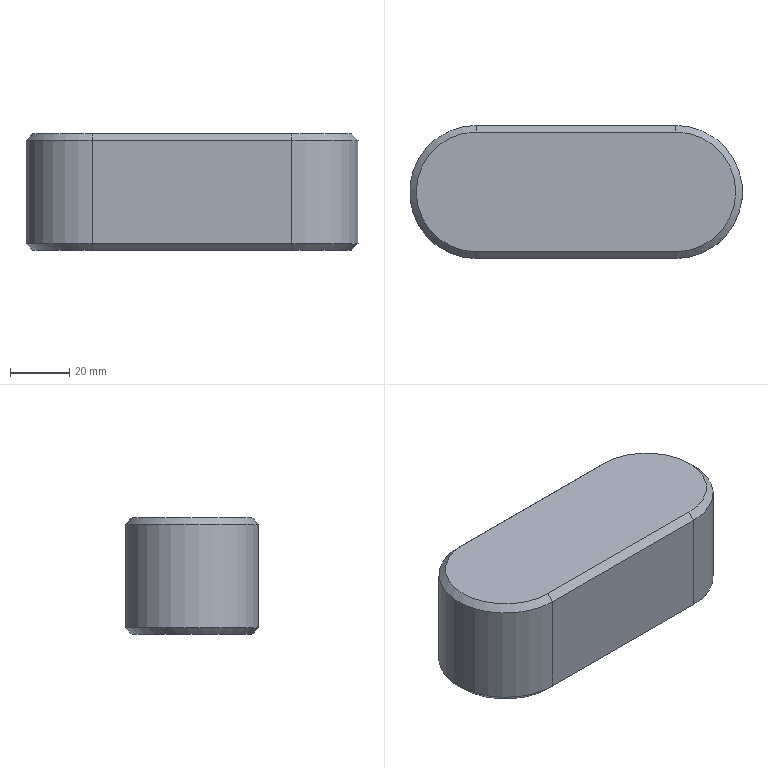Part | NX | features 28.SLDPRT 2, Delete Body 1, LINKED_BODY 1, SCALE 1 | 1 solid | 14 faces | box 112.5 x 45 x 39.375 mm | volume 180850 mm3 | plane 8 | cone 4 | cylinder 2 | commonest cylinder face diameters 45 x2
STEP:
#1=CARTESIAN_POINT('',(-34.875,-1747.479,329.645));
#2=VERTEX_POINT('',#1);
#3=CARTESIAN_POINT('',(-34.875,-1747.479,294.77));
#4=VERTEX_POINT('',#3);
#5=CARTESIAN_POINT('',(-34.875,-1747.479,331.895));
#6=DIRECTION('',(0.,0.,-1.));
#7=VECTOR('',#6,1000.);
#8=LINE('',#5,#7);
#9=EDGE_CURVE('',#2,#4,#8,.T.);
#10=ORIENTED_EDGE('',*,*,#9,.F.);
#11=CARTESIAN_POINT('',(-34.875,-1702.479,329.645));
#12=VERTEX_POINT('',#11);
#13=CARTESIAN_POINT('',(-34.875,-1724.979,329.645));
#14=DIRECTION('',(0.,0.,-1.));
#15=DIRECTION('',(-1.,0.,0.));
#16=AXIS2_PLACEMENT_3D('',#13,#14,#15);
#17=CIRCLE('',#16,22.5);
#18=EDGE_CURVE('',#2,#12,#17,.T.);
#19=ORIENTED_EDGE('',*,*,#18,.T.);
#20=CARTESIAN_POINT('',(-34.875,-1702.479,294.77));
#21=VERTEX_POINT('',#20);
#22=CARTESIAN_POINT('',(-34.875,-1702.479,331.895));
#23=DIRECTION('',(0.,0.,-1.));
#24=VECTOR('',#23,1000.);
#25=LINE('',#22,#24);
#26=EDGE_CURVE('',#12,#21,#25,.T.);
#27=ORIENTED_EDGE('',*,*,#26,.T.);
#28=CARTESIAN_POINT('',(-34.875,-1724.979,294.77));
#29=DIRECTION('',(0.,0.,-1.));
#30=DIRECTION('',(-1.,0.,0.));
#31=AXIS2_PLACEMENT_3D('',#28,#29,#30);
#32=CIRCLE('',#31,22.5);
#33=EDGE_CURVE('',#21,#4,#32,.F.);
#34=ORIENTED_EDGE('',*,*,#33,.T.);
#35=EDGE_LOOP('',(#10,#19,#27,#34));
#36=FACE_BOUND('',#35,.T.);
#37=CARTESIAN_POINT('',(-34.875,-1724.979,331.895));
#38=DIRECTION('',(0.,0.,-1.));
#39=DIRECTION('',(-1.,0.,0.));
#40=AXIS2_PLACEMENT_3D('',#37,#38,#39);
#41=CYLINDRICAL_SURFACE('',#40,22.5);
#42=ADVANCED_FACE('',(#36),#41,.T.);
#43=ORIENTED_EDGE('',*,*,#9,.T.);
#44=CARTESIAN_POINT('',(32.625,-1747.479,294.77));
#45=VERTEX_POINT('',#44);
#46=CARTESIAN_POINT('',(32.625,-1747.479,294.77));
#47=DIRECTION('',(1.,0.,0.));
#48=VECTOR('',#47,1000.);
#49=LINE('',#46,#48);
#50=EDGE_CURVE('',#4,#45,#49,.T.);
#51=ORIENTED_EDGE('',*,*,#50,.T.);
#52=CARTESIAN_POINT('',(32.625,-1747.479,329.645));
#53=VERTEX_POINT('',#52);
#54=CARTESIAN_POINT('',(32.625,-1747.479,331.895));
#55=DIRECTION('',(0.,0.,-1.));
#56=VECTOR('',#55,1000.);
#57=LINE('',#54,#56);
#58=EDGE_CURVE('',#53,#45,#57,.T.);
#59=ORIENTED_EDGE('',*,*,#58,.F.);
#60=CARTESIAN_POINT('',(32.625,-1747.479,329.645));
#61=DIRECTION('',(-1.,0.,0.));
#62=VECTOR('',#61,1000.);
#63=LINE('',#60,#62);
#64=EDGE_CURVE('',#53,#2,#63,.T.);
#65=ORIENTED_EDGE('',*,*,#64,.T.);
#66=EDGE_LOOP('',(#43,#51,#59,#65));
#67=FACE_BOUND('',#66,.T.);
#68=CARTESIAN_POINT('',(32.625,-1747.479,331.895));
#69=DIRECTION('',(0.,1.,0.));
#70=DIRECTION('',(-1.,0.,0.));
#71=AXIS2_PLACEMENT_3D('',#68,#69,#70);
#72=PLANE('',#71);
#73=ADVANCED_FACE('',(#67),#72,.F.);
#74=CARTESIAN_POINT('',(32.625,-1702.479,329.645));
#75=VERTEX_POINT('',#74);
#76=CARTESIAN_POINT('',(32.625,-1702.479,294.77));
#77=VERTEX_POINT('',#76);
#78=CARTESIAN_POINT('',(32.625,-1702.479,331.895));
#79=DIRECTION('',(0.,0.,-1.));
#80=VECTOR('',#79,1000.);
#81=LINE('',#78,#80);
#82=EDGE_CURVE('',#75,#77,#81,.T.);
#83=ORIENTED_EDGE('',*,*,#82,.F.);
#84=CARTESIAN_POINT('',(32.625,-1724.979,329.645));
#85=DIRECTION('',(0.,0.,-1.));
#86=DIRECTION('',(-1.,0.,0.));
#87=AXIS2_PLACEMENT_3D('',#84,#85,#86);
#88=CIRCLE('',#87,22.5);
#89=EDGE_CURVE('',#75,#53,#88,.T.);
#90=ORIENTED_EDGE('',*,*,#89,.T.);
#91=ORIENTED_EDGE('',*,*,#58,.T.);
#92=CARTESIAN_POINT('',(32.625,-1724.979,294.77));
#93=DIRECTION('',(0.,0.,-1.));
#94=DIRECTION('',(-1.,0.,0.));
#95=AXIS2_PLACEMENT_3D('',#92,#93,#94);
#96=CIRCLE('',#95,22.5);
#97=EDGE_CURVE('',#45,#77,#96,.F.);
#98=ORIENTED_EDGE('',*,*,#97,.T.);
#99=EDGE_LOOP('',(#83,#90,#91,#98));
#100=FACE_BOUND('',#99,.T.);
#101=CARTESIAN_POINT('',(32.625,-1724.979,331.895));
#102=DIRECTION('',(0.,0.,-1.));
#103=DIRECTION('',(-1.,0.,0.));
#104=AXIS2_PLACEMENT_3D('',#101,#102,#103);
#105=CYLINDRICAL_SURFACE('',#104,22.5);
#106=ADVANCED_FACE('',(#100),#105,.T.);
#107=ORIENTED_EDGE('',*,*,#26,.F.);
#108=CARTESIAN_POINT('',(-34.875,-1702.479,329.645));
#109=DIRECTION('',(1.,0.,0.));
#110=VECTOR('',#109,1000.);
#111=LINE('',#108,#110);
#112=EDGE_CURVE('',#12,#75,#111,.T.);
#113=ORIENTED_EDGE('',*,*,#112,.T.);
#114=ORIENTED_EDGE('',*,*,#82,.T.);
#115=CARTESIAN_POINT('',(-34.875,-1702.479,294.77));
#116=DIRECTION('',(-1.,0.,0.));
#117=VECTOR('',#116,1000.);
#118=LINE('',#115,#117);
#119=EDGE_CURVE('',#77,#21,#118,.T.);
#120=ORIENTED_EDGE('',*,*,#119,.T.);
#121=EDGE_LOOP('',(#107,#113,#114,#120));
#122=FACE_BOUND('',#121,.T.);
#123=CARTESIAN_POINT('',(-34.875,-1702.479,331.895));
#124=DIRECTION('',(0.,-1.,0.));
#125=DIRECTION('',(0.,0.,-1.));
#126=AXIS2_PLACEMENT_3D('',#123,#124,#125);
#127=PLANE('',#126);
#128=ADVANCED_FACE('',(#122),#127,.F.);
#129=CARTESIAN_POINT('',(-34.875,-1704.729,331.895));
#130=VERTEX_POINT('',#129);
#131=CARTESIAN_POINT('',(-34.875,-1745.229,331.895));
#132=VERTEX_POINT('',#131);
#133=CARTESIAN_POINT('',(-34.875,-1724.979,331.895));
#134=DIRECTION('',(0.,0.,-1.));
#135=DIRECTION('',(-1.,0.,0.));
#136=AXIS2_PLACEMENT_3D('',#133,#134,#135);
#137=CIRCLE('',#136,20.25);
#138=EDGE_CURVE('',#130,#132,#137,.F.);
#139=ORIENTED_EDGE('',*,*,#138,.T.);
#140=CARTESIAN_POINT('',(32.625,-1745.229,331.895));
#141=VERTEX_POINT('',#140);
#142=CARTESIAN_POINT('',(-34.875,-1745.229,331.895));
#143=DIRECTION('',(1.,0.,0.));
#144=VECTOR('',#143,1000.);
#145=LINE('',#142,#144);
#146=EDGE_CURVE('',#132,#141,#145,.T.);
#147=ORIENTED_EDGE('',*,*,#146,.T.);
#148=CARTESIAN_POINT('',(32.625,-1704.729,331.895));
#149=VERTEX_POINT('',#148);
#150=CARTESIAN_POINT('',(32.625,-1724.979,331.895));
#151=DIRECTION('',(0.,0.,-1.));
#152=DIRECTION('',(-1.,0.,0.));
#153=AXIS2_PLACEMENT_3D('',#150,#151,#152);
#154=CIRCLE('',#153,20.25);
#155=EDGE_CURVE('',#141,#149,#154,.F.);
#156=ORIENTED_EDGE('',*,*,#155,.T.);
#157=CARTESIAN_POINT('',(-34.875,-1704.729,331.895));
#158=DIRECTION('',(-1.,0.,0.));
#159=VECTOR('',#158,1000.);
#160=LINE('',#157,#159);
#161=EDGE_CURVE('',#149,#130,#160,.T.);
#162=ORIENTED_EDGE('',*,*,#161,.T.);
#163=EDGE_LOOP('',(#139,#147,#156,#162));
#164=FACE_BOUND('',#163,.T.);
#165=CARTESIAN_POINT('',(-34.875,-1724.979,331.895));
#166=DIRECTION('',(0.,0.,-1.));
#167=DIRECTION('',(-1.,0.,0.));
#168=AXIS2_PLACEMENT_3D('',#165,#166,#167);
#169=PLANE('',#168);
#170=ADVANCED_FACE('',(#164),#169,.F.);
#171=CARTESIAN_POINT('',(32.625,-1704.729,292.52));
#172=VERTEX_POINT('',#171);
#173=CARTESIAN_POINT('',(32.625,-1745.229,292.52));
#174=VERTEX_POINT('',#173);
#175=CARTESIAN_POINT('',(32.625,-1724.979,292.52));
#176=DIRECTION('',(0.,0.,-1.));
#177=DIRECTION('',(-1.,0.,0.));
#178=AXIS2_PLACEMENT_3D('',#175,#176,#177);
#179=CIRCLE('',#178,20.25);
#180=EDGE_CURVE('',#172,#174,#179,.T.);
#181=ORIENTED_EDGE('',*,*,#180,.T.);
#182=CARTESIAN_POINT('',(-34.875,-1745.229,292.52));
#183=VERTEX_POINT('',#182);
#184=CARTESIAN_POINT('',(-34.875,-1745.229,292.52));
#185=DIRECTION('',(-1.,0.,0.));
#186=VECTOR('',#185,1000.);
#187=LINE('',#184,#186);
#188=EDGE_CURVE('',#174,#183,#187,.T.);
#189=ORIENTED_EDGE('',*,*,#188,.T.);
#190=CARTESIAN_POINT('',(-34.875,-1704.729,292.52));
#191=VERTEX_POINT('',#190);
#192=CARTESIAN_POINT('',(-34.875,-1724.979,292.52));
#193=DIRECTION('',(0.,0.,-1.));
#194=DIRECTION('',(-1.,0.,0.));
#195=AXIS2_PLACEMENT_3D('',#192,#193,#194);
#196=CIRCLE('',#195,20.25);
#197=EDGE_CURVE('',#183,#191,#196,.T.);
#198=ORIENTED_EDGE('',*,*,#197,.T.);
#199=CARTESIAN_POINT('',(32.625,-1704.729,292.52));
#200=DIRECTION('',(1.,0.,0.));
#201=VECTOR('',#200,1000.);
#202=LINE('',#199,#201);
#203=EDGE_CURVE('',#191,#172,#202,.T.);
#204=ORIENTED_EDGE('',*,*,#203,.T.);
#205=EDGE_LOOP('',(#181,#189,#198,#204));
#206=FACE_BOUND('',#205,.T.);
#207=CARTESIAN_POINT('',(-34.875,-1724.979,292.52));
#208=DIRECTION('',(0.,0.,-1.));
#209=DIRECTION('',(-1.,0.,0.));
#210=AXIS2_PLACEMENT_3D('',#207,#208,#209);
#211=PLANE('',#210);
#212=ADVANCED_FACE('',(#206),#211,.T.);
#213=CARTESIAN_POINT('',(32.625,-1704.729,292.52));
#214=DIRECTION('',(0.,0.7071,0.7071));
#215=VECTOR('',#214,1000.);
#216=LINE('',#213,#215);
#217=EDGE_CURVE('',#172,#77,#216,.T.);
#218=ORIENTED_EDGE('',*,*,#217,.F.);
#219=ORIENTED_EDGE('',*,*,#203,.F.);
#220=CARTESIAN_POINT('',(-34.875,-1702.479,294.77));
#221=DIRECTION('',(0.,-0.7071,-0.7071));
#222=VECTOR('',#221,1000.);
#223=LINE('',#220,#222);
#224=EDGE_CURVE('',#21,#191,#223,.T.);
#225=ORIENTED_EDGE('',*,*,#224,.F.);
#226=ORIENTED_EDGE('',*,*,#119,.F.);
#227=EDGE_LOOP('',(#218,#219,#225,#226));
#228=FACE_BOUND('',#227,.T.);
#229=CARTESIAN_POINT('',(-34.875,-1702.479,294.77));
#230=DIRECTION('',(0.,0.7071,-0.7071));
#231=DIRECTION('',(0.,0.7071,0.7071));
#232=AXIS2_PLACEMENT_3D('',#229,#230,#231);
#233=PLANE('',#232);
#234=ADVANCED_FACE('',(#228),#233,.T.);
#235=ORIENTED_EDGE('',*,*,#224,.T.);
#236=ORIENTED_EDGE('',*,*,#197,.F.);
#237=CARTESIAN_POINT('',(-34.875,-1747.479,294.77));
#238=DIRECTION('',(0.,0.7071,-0.7071));
#239=VECTOR('',#238,1000.);
#240=LINE('',#237,#239);
#241=EDGE_CURVE('',#4,#183,#240,.T.);
#242=ORIENTED_EDGE('',*,*,#241,.F.);
#243=ORIENTED_EDGE('',*,*,#33,.F.);
#244=EDGE_LOOP('',(#235,#236,#242,#243));
#245=FACE_BOUND('',#244,.T.);
#246=CARTESIAN_POINT('',(-34.875,-1724.979,294.77));
#247=DIRECTION('',(0.,0.,1.));
#248=DIRECTION('',(1.,0.,0.));
#249=AXIS2_PLACEMENT_3D('',#246,#247,#248);
#250=CONICAL_SURFACE('',#249,22.5,0.7854);
#251=ADVANCED_FACE('',(#245),#250,.T.);
#252=ORIENTED_EDGE('',*,*,#217,.T.);
#253=ORIENTED_EDGE('',*,*,#97,.F.);
#254=CARTESIAN_POINT('',(32.625,-1745.229,292.52));
#255=DIRECTION('',(0.,-0.7071,0.7071));
#256=VECTOR('',#255,1000.);
#257=LINE('',#254,#256);
#258=EDGE_CURVE('',#174,#45,#257,.T.);
#259=ORIENTED_EDGE('',*,*,#258,.F.);
#260=ORIENTED_EDGE('',*,*,#180,.F.);
#261=EDGE_LOOP('',(#252,#253,#259,#260));
#262=FACE_BOUND('',#261,.T.);
#263=CARTESIAN_POINT('',(32.625,-1724.979,294.77));
#264=DIRECTION('',(0.,0.,1.));
#265=DIRECTION('',(1.,0.,0.));
#266=AXIS2_PLACEMENT_3D('',#263,#264,#265);
#267=CONICAL_SURFACE('',#266,22.5,0.7854);
#268=ADVANCED_FACE('',(#262),#267,.T.);
#269=ORIENTED_EDGE('',*,*,#241,.T.);
#270=ORIENTED_EDGE('',*,*,#188,.F.);
#271=ORIENTED_EDGE('',*,*,#258,.T.);
#272=ORIENTED_EDGE('',*,*,#50,.F.);
#273=EDGE_LOOP('',(#269,#270,#271,#272));
#274=FACE_BOUND('',#273,.T.);
#275=CARTESIAN_POINT('',(32.625,-1747.479,294.77));
#276=DIRECTION('',(0.,-0.7071,-0.7071));
#277=DIRECTION('',(0.,0.7071,-0.7071));
#278=AXIS2_PLACEMENT_3D('',#275,#276,#277);
#279=PLANE('',#278);
#280=ADVANCED_FACE('',(#274),#279,.T.);
#281=CARTESIAN_POINT('',(32.625,-1702.479,329.645));
#282=DIRECTION('',(0.,-0.7071,0.7071));
#283=VECTOR('',#282,1000.);
#284=LINE('',#281,#283);
#285=EDGE_CURVE('',#75,#149,#284,.T.);
#286=ORIENTED_EDGE('',*,*,#285,.F.);
#287=ORIENTED_EDGE('',*,*,#112,.F.);
#288=CARTESIAN_POINT('',(-34.875,-1704.729,331.895));
#289=DIRECTION('',(0.,0.7071,-0.7071));
#290=VECTOR('',#289,1000.);
#291=LINE('',#288,#290);
#292=EDGE_CURVE('',#130,#12,#291,.T.);
#293=ORIENTED_EDGE('',*,*,#292,.F.);
#294=ORIENTED_EDGE('',*,*,#161,.F.);
#295=EDGE_LOOP('',(#286,#287,#293,#294));
#296=FACE_BOUND('',#295,.T.);
#297=CARTESIAN_POINT('',(-34.875,-1704.729,331.895));
#298=DIRECTION('',(0.,-0.7071,-0.7071));
#299=DIRECTION('',(0.,0.7071,-0.7071));
#300=AXIS2_PLACEMENT_3D('',#297,#298,#299);
#301=PLANE('',#300);
#302=ADVANCED_FACE('',(#296),#301,.F.);
#303=ORIENTED_EDGE('',*,*,#292,.T.);
#304=ORIENTED_EDGE('',*,*,#18,.F.);
#305=CARTESIAN_POINT('',(-34.875,-1745.229,331.895));
#306=DIRECTION('',(0.,-0.7071,-0.7071));
#307=VECTOR('',#306,1000.);
#308=LINE('',#305,#307);
#309=EDGE_CURVE('',#132,#2,#308,.T.);
#310=ORIENTED_EDGE('',*,*,#309,.F.);
#311=ORIENTED_EDGE('',*,*,#138,.F.);
#312=EDGE_LOOP('',(#303,#304,#310,#311));
#313=FACE_BOUND('',#312,.T.);
#314=CARTESIAN_POINT('',(-34.875,-1724.979,331.895));
#315=DIRECTION('',(0.,0.,-1.));
#316=DIRECTION('',(-1.,0.,0.));
#317=AXIS2_PLACEMENT_3D('',#314,#315,#316);
#318=CONICAL_SURFACE('',#317,20.25,0.7854);
#319=ADVANCED_FACE('',(#313),#318,.T.);
#320=ORIENTED_EDGE('',*,*,#285,.T.);
#321=ORIENTED_EDGE('',*,*,#155,.F.);
#322=CARTESIAN_POINT('',(32.625,-1747.479,329.645));
#323=DIRECTION('',(0.,0.7071,0.7071));
#324=VECTOR('',#323,1000.);
#325=LINE('',#322,#324);
#326=EDGE_CURVE('',#53,#141,#325,.T.);
#327=ORIENTED_EDGE('',*,*,#326,.F.);
#328=ORIENTED_EDGE('',*,*,#89,.F.);
#329=EDGE_LOOP('',(#320,#321,#327,#328));
#330=FACE_BOUND('',#329,.T.);
#331=CARTESIAN_POINT('',(32.625,-1724.979,331.895));
#332=DIRECTION('',(0.,0.,-1.));
#333=DIRECTION('',(-1.,0.,0.));
#334=AXIS2_PLACEMENT_3D('',#331,#332,#333);
#335=CONICAL_SURFACE('',#334,20.25,0.7854);
#336=ADVANCED_FACE('',(#330),#335,.T.);
#337=ORIENTED_EDGE('',*,*,#309,.T.);
#338=ORIENTED_EDGE('',*,*,#64,.F.);
#339=ORIENTED_EDGE('',*,*,#326,.T.);
#340=ORIENTED_EDGE('',*,*,#146,.F.);
#341=EDGE_LOOP('',(#337,#338,#339,#340));
#342=FACE_BOUND('',#341,.T.);
#343=CARTESIAN_POINT('',(-34.875,-1745.229,331.895));
#344=DIRECTION('',(0.,0.7071,-0.7071));
#345=DIRECTION('',(0.,0.7071,0.7071));
#346=AXIS2_PLACEMENT_3D('',#343,#344,#345);
#347=PLANE('',#346);
#348=ADVANCED_FACE('',(#342),#347,.F.);
#349=CLOSED_SHELL('',(#42,#73,#106,#128,#170,#212,#234,#251,#268,#280,#302,#319,#336,#348));
#350=MANIFOLD_SOLID_BREP('',#349);
#351=(LENGTH_UNIT()NAMED_UNIT(*)SI_UNIT(.MILLI.,.METRE.));
#352=UNCERTAINTY_MEASURE_WITH_UNIT(LENGTH_MEASURE(0.00001),#351,'','');
#353=(NAMED_UNIT(*)PLANE_ANGLE_UNIT()SI_UNIT($,.RADIAN.));
#354=(NAMED_UNIT(*)SI_UNIT($,.STERADIAN.)SOLID_ANGLE_UNIT());
#355=(GEOMETRIC_REPRESENTATION_CONTEXT(3)GLOBAL_UNCERTAINTY_ASSIGNED_CONTEXT((#352))GLOBAL_UNIT_ASSIGNED_CONTEXT((#351,#353,#354))REPRESENTATION_CONTEXT('',''));
#356=ADVANCED_BREP_SHAPE_REPRESENTATION('',(#350),#355);